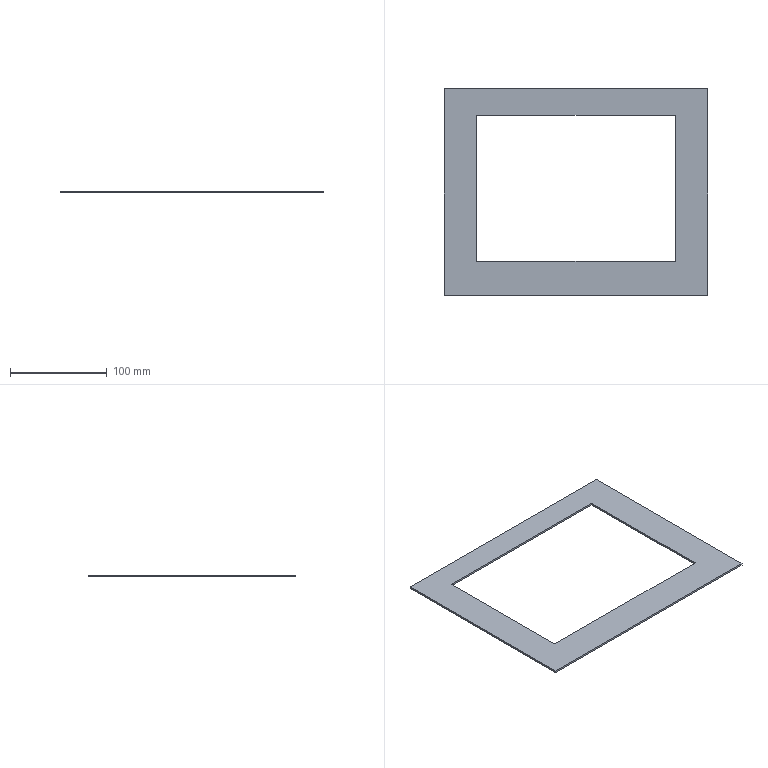Part | STEP file | Front guard plate SGN-7-05 | 1 solid | 10 faces | box 272 x 213 x 2 mm | volume 53962 mm3 | plane 10
STEP:
#1=CARTESIAN_POINT('',(0.,0.,0.));
#2=DIRECTION('',(0.,0.,1.));
#3=DIRECTION('',(1.,0.,0.));
#4=AXIS2_PLACEMENT_3D('',#1,#2,#3);
#5=CARTESIAN_POINT('',(136.,-106.5,0.));
#6=VERTEX_POINT('',#5);
#7=CARTESIAN_POINT('',(136.,106.5,0.));
#8=VERTEX_POINT('',#7);
#9=CARTESIAN_POINT('',(136.,-106.5,0.));
#10=DIRECTION('',(0.,1.,0.));
#11=VECTOR('',#10,1.);
#12=LINE('',#9,#11);
#13=CARTESIAN_POINT('',(136.,-106.5,-2.));
#14=DIRECTION('',(1.,0.,0.));
#15=DIRECTION('',(0.,0.,-1.));
#16=AXIS2_PLACEMENT_3D('',#13,#14,#15);
#17=PLANE('',#16);
#18=CARTESIAN_POINT('',(-2.,0.));
#19=DIRECTION('',(0.,1.));
#20=VECTOR('',#19,1.);
#21=LINE('',#18,#20);
#22=(GEOMETRIC_REPRESENTATION_CONTEXT(2)PARAMETRIC_REPRESENTATION_CONTEXT()REPRESENTATION_CONTEXT('',''));
#23=DEFINITIONAL_REPRESENTATION('',(#21),#22);
#24=PCURVE('',#17,#23);
#25=CARTESIAN_POINT('',(0.,0.,0.));
#26=DIRECTION('',(0.,0.,-1.));
#27=DIRECTION('',(-1.,0.,0.));
#28=AXIS2_PLACEMENT_3D('',#25,#26,#27);
#29=PLANE('',#28);
#30=CARTESIAN_POINT('',(-136.,-106.5));
#31=DIRECTION('',(0.,1.));
#32=VECTOR('',#31,1.);
#33=LINE('',#30,#32);
#34=(GEOMETRIC_REPRESENTATION_CONTEXT(2)PARAMETRIC_REPRESENTATION_CONTEXT()REPRESENTATION_CONTEXT('',''));
#35=DEFINITIONAL_REPRESENTATION('',(#33),#34);
#36=PCURVE('',#29,#35);
#37=SURFACE_CURVE('',#12,(#24,#36),.PCURVE_S1.);
#38=EDGE_CURVE('',#6,#8,#37,.T.);
#39=ORIENTED_EDGE('',*,*,#38,.F.);
#40=CARTESIAN_POINT('',(136.,-106.5,-2.));
#41=VERTEX_POINT('',#40);
#42=CARTESIAN_POINT('',(136.,-106.5,-2.));
#43=DIRECTION('',(0.,0.,1.));
#44=VECTOR('',#43,1.);
#45=LINE('',#42,#44);
#46=CARTESIAN_POINT('',(0.,0.));
#47=DIRECTION('',(-1.,0.));
#48=VECTOR('',#47,1.);
#49=LINE('',#46,#48);
#50=(GEOMETRIC_REPRESENTATION_CONTEXT(2)PARAMETRIC_REPRESENTATION_CONTEXT()REPRESENTATION_CONTEXT('',''));
#51=DEFINITIONAL_REPRESENTATION('',(#49),#50);
#52=PCURVE('',#17,#51);
#53=CARTESIAN_POINT('',(-136.,-106.5,-2.));
#54=DIRECTION('',(0.,-1.,0.));
#55=DIRECTION('',(0.,0.,-1.));
#56=AXIS2_PLACEMENT_3D('',#53,#54,#55);
#57=PLANE('',#56);
#58=CARTESIAN_POINT('',(0.,272.));
#59=DIRECTION('',(-1.,0.));
#60=VECTOR('',#59,1.);
#61=LINE('',#58,#60);
#62=(GEOMETRIC_REPRESENTATION_CONTEXT(2)PARAMETRIC_REPRESENTATION_CONTEXT()REPRESENTATION_CONTEXT('',''));
#63=DEFINITIONAL_REPRESENTATION('',(#61),#62);
#64=PCURVE('',#57,#63);
#65=SURFACE_CURVE('',#45,(#52,#64),.PCURVE_S1.);
#66=EDGE_CURVE('',#41,#6,#65,.T.);
#67=ORIENTED_EDGE('',*,*,#66,.F.);
#68=CARTESIAN_POINT('',(136.,106.5,-2.));
#69=VERTEX_POINT('',#68);
#70=CARTESIAN_POINT('',(136.,-106.5,-2.));
#71=DIRECTION('',(0.,1.,0.));
#72=VECTOR('',#71,1.);
#73=LINE('',#70,#72);
#74=CARTESIAN_POINT('',(0.,0.));
#75=DIRECTION('',(0.,1.));
#76=VECTOR('',#75,1.);
#77=LINE('',#74,#76);
#78=(GEOMETRIC_REPRESENTATION_CONTEXT(2)PARAMETRIC_REPRESENTATION_CONTEXT()REPRESENTATION_CONTEXT('',''));
#79=DEFINITIONAL_REPRESENTATION('',(#77),#78);
#80=PCURVE('',#17,#79);
#81=CARTESIAN_POINT('',(0.,0.,-2.));
#82=DIRECTION('',(0.,0.,-1.));
#83=DIRECTION('',(-1.,0.,0.));
#84=AXIS2_PLACEMENT_3D('',#81,#82,#83);
#85=PLANE('',#84);
#86=CARTESIAN_POINT('',(-136.,-106.5));
#87=DIRECTION('',(0.,1.));
#88=VECTOR('',#87,1.);
#89=LINE('',#86,#88);
#90=(GEOMETRIC_REPRESENTATION_CONTEXT(2)PARAMETRIC_REPRESENTATION_CONTEXT()REPRESENTATION_CONTEXT('',''));
#91=DEFINITIONAL_REPRESENTATION('',(#89),#90);
#92=PCURVE('',#85,#91);
#93=SURFACE_CURVE('',#73,(#80,#92),.PCURVE_S1.);
#94=EDGE_CURVE('',#41,#69,#93,.T.);
#95=ORIENTED_EDGE('',*,*,#94,.T.);
#96=CARTESIAN_POINT('',(136.,106.5,-2.));
#97=DIRECTION('',(0.,0.,1.));
#98=VECTOR('',#97,1.);
#99=LINE('',#96,#98);
#100=CARTESIAN_POINT('',(0.,213.));
#101=DIRECTION('',(-1.,0.));
#102=VECTOR('',#101,1.);
#103=LINE('',#100,#102);
#104=(GEOMETRIC_REPRESENTATION_CONTEXT(2)PARAMETRIC_REPRESENTATION_CONTEXT()REPRESENTATION_CONTEXT('',''));
#105=DEFINITIONAL_REPRESENTATION('',(#103),#104);
#106=PCURVE('',#17,#105);
#107=CARTESIAN_POINT('',(-136.,106.5,-2.));
#108=DIRECTION('',(0.,1.,0.));
#109=DIRECTION('',(0.,0.,1.));
#110=AXIS2_PLACEMENT_3D('',#107,#108,#109);
#111=PLANE('',#110);
#112=CARTESIAN_POINT('',(0.,272.));
#113=DIRECTION('',(1.,0.));
#114=VECTOR('',#113,1.);
#115=LINE('',#112,#114);
#116=(GEOMETRIC_REPRESENTATION_CONTEXT(2)PARAMETRIC_REPRESENTATION_CONTEXT()REPRESENTATION_CONTEXT('',''));
#117=DEFINITIONAL_REPRESENTATION('',(#115),#116);
#118=PCURVE('',#111,#117);
#119=SURFACE_CURVE('',#99,(#106,#118),.PCURVE_S1.);
#120=EDGE_CURVE('',#69,#8,#119,.T.);
#121=ORIENTED_EDGE('',*,*,#120,.T.);
#122=EDGE_LOOP('',(#39,#67,#95,#121));
#123=FACE_BOUND('',#122,.T.);
#124=ADVANCED_FACE('',(#123),#17,.T.);
#125=CARTESIAN_POINT('',(-136.,-106.5,0.));
#126=VERTEX_POINT('',#125);
#127=CARTESIAN_POINT('',(-136.,-106.5,0.));
#128=DIRECTION('',(1.,0.,0.));
#129=VECTOR('',#128,1.);
#130=LINE('',#127,#129);
#131=CARTESIAN_POINT('',(-2.,0.));
#132=DIRECTION('',(0.,1.));
#133=VECTOR('',#132,1.);
#134=LINE('',#131,#133);
#135=(GEOMETRIC_REPRESENTATION_CONTEXT(2)PARAMETRIC_REPRESENTATION_CONTEXT()REPRESENTATION_CONTEXT('',''));
#136=DEFINITIONAL_REPRESENTATION('',(#134),#135);
#137=PCURVE('',#57,#136);
#138=CARTESIAN_POINT('',(136.,-106.5));
#139=DIRECTION('',(-1.,0.));
#140=VECTOR('',#139,1.);
#141=LINE('',#138,#140);
#142=(GEOMETRIC_REPRESENTATION_CONTEXT(2)PARAMETRIC_REPRESENTATION_CONTEXT()REPRESENTATION_CONTEXT('',''));
#143=DEFINITIONAL_REPRESENTATION('',(#141),#142);
#144=PCURVE('',#29,#143);
#145=SURFACE_CURVE('',#130,(#137,#144),.PCURVE_S1.);
#146=EDGE_CURVE('',#126,#6,#145,.T.);
#147=ORIENTED_EDGE('',*,*,#146,.F.);
#148=CARTESIAN_POINT('',(-136.,-106.5,-2.));
#149=VERTEX_POINT('',#148);
#150=CARTESIAN_POINT('',(-136.,-106.5,-2.));
#151=DIRECTION('',(0.,0.,1.));
#152=VECTOR('',#151,1.);
#153=LINE('',#150,#152);
#154=CARTESIAN_POINT('',(0.,0.));
#155=DIRECTION('',(-1.,0.));
#156=VECTOR('',#155,1.);
#157=LINE('',#154,#156);
#158=(GEOMETRIC_REPRESENTATION_CONTEXT(2)PARAMETRIC_REPRESENTATION_CONTEXT()REPRESENTATION_CONTEXT('',''));
#159=DEFINITIONAL_REPRESENTATION('',(#157),#158);
#160=PCURVE('',#57,#159);
#161=CARTESIAN_POINT('',(-136.,-106.5,-2.));
#162=DIRECTION('',(-1.,0.,0.));
#163=DIRECTION('',(0.,0.,1.));
#164=AXIS2_PLACEMENT_3D('',#161,#162,#163);
#165=PLANE('',#164);
#166=CARTESIAN_POINT('',(0.,0.));
#167=DIRECTION('',(1.,0.));
#168=VECTOR('',#167,1.);
#169=LINE('',#166,#168);
#170=(GEOMETRIC_REPRESENTATION_CONTEXT(2)PARAMETRIC_REPRESENTATION_CONTEXT()REPRESENTATION_CONTEXT('',''));
#171=DEFINITIONAL_REPRESENTATION('',(#169),#170);
#172=PCURVE('',#165,#171);
#173=SURFACE_CURVE('',#153,(#160,#172),.PCURVE_S1.);
#174=EDGE_CURVE('',#149,#126,#173,.T.);
#175=ORIENTED_EDGE('',*,*,#174,.F.);
#176=CARTESIAN_POINT('',(-136.,-106.5,-2.));
#177=DIRECTION('',(1.,0.,0.));
#178=VECTOR('',#177,1.);
#179=LINE('',#176,#178);
#180=CARTESIAN_POINT('',(0.,0.));
#181=DIRECTION('',(0.,1.));
#182=VECTOR('',#181,1.);
#183=LINE('',#180,#182);
#184=(GEOMETRIC_REPRESENTATION_CONTEXT(2)PARAMETRIC_REPRESENTATION_CONTEXT()REPRESENTATION_CONTEXT('',''));
#185=DEFINITIONAL_REPRESENTATION('',(#183),#184);
#186=PCURVE('',#57,#185);
#187=CARTESIAN_POINT('',(136.,-106.5));
#188=DIRECTION('',(-1.,0.));
#189=VECTOR('',#188,1.);
#190=LINE('',#187,#189);
#191=(GEOMETRIC_REPRESENTATION_CONTEXT(2)PARAMETRIC_REPRESENTATION_CONTEXT()REPRESENTATION_CONTEXT('',''));
#192=DEFINITIONAL_REPRESENTATION('',(#190),#191);
#193=PCURVE('',#85,#192);
#194=SURFACE_CURVE('',#179,(#186,#193),.PCURVE_S1.);
#195=EDGE_CURVE('',#149,#41,#194,.T.);
#196=ORIENTED_EDGE('',*,*,#195,.T.);
#197=ORIENTED_EDGE('',*,*,#66,.T.);
#198=EDGE_LOOP('',(#147,#175,#196,#197));
#199=FACE_BOUND('',#198,.T.);
#200=ADVANCED_FACE('',(#199),#57,.T.);
#201=CARTESIAN_POINT('',(-136.,106.5,0.));
#202=VERTEX_POINT('',#201);
#203=CARTESIAN_POINT('',(-136.,-106.5,0.));
#204=DIRECTION('',(0.,-1.,0.));
#205=VECTOR('',#204,1.);
#206=LINE('',#203,#205);
#207=CARTESIAN_POINT('',(2.,0.));
#208=DIRECTION('',(0.,-1.));
#209=VECTOR('',#208,1.);
#210=LINE('',#207,#209);
#211=(GEOMETRIC_REPRESENTATION_CONTEXT(2)PARAMETRIC_REPRESENTATION_CONTEXT()REPRESENTATION_CONTEXT('',''));
#212=DEFINITIONAL_REPRESENTATION('',(#210),#211);
#213=PCURVE('',#165,#212);
#214=CARTESIAN_POINT('',(136.,-106.5));
#215=DIRECTION('',(0.,-1.));
#216=VECTOR('',#215,1.);
#217=LINE('',#214,#216);
#218=(GEOMETRIC_REPRESENTATION_CONTEXT(2)PARAMETRIC_REPRESENTATION_CONTEXT()REPRESENTATION_CONTEXT('',''));
#219=DEFINITIONAL_REPRESENTATION('',(#217),#218);
#220=PCURVE('',#29,#219);
#221=SURFACE_CURVE('',#206,(#213,#220),.PCURVE_S1.);
#222=EDGE_CURVE('',#202,#126,#221,.T.);
#223=ORIENTED_EDGE('',*,*,#222,.F.);
#224=CARTESIAN_POINT('',(-136.,106.5,-2.));
#225=VERTEX_POINT('',#224);
#226=CARTESIAN_POINT('',(-136.,106.5,-2.));
#227=DIRECTION('',(0.,0.,1.));
#228=VECTOR('',#227,1.);
#229=LINE('',#226,#228);
#230=CARTESIAN_POINT('',(0.,213.));
#231=DIRECTION('',(1.,0.));
#232=VECTOR('',#231,1.);
#233=LINE('',#230,#232);
#234=(GEOMETRIC_REPRESENTATION_CONTEXT(2)PARAMETRIC_REPRESENTATION_CONTEXT()REPRESENTATION_CONTEXT('',''));
#235=DEFINITIONAL_REPRESENTATION('',(#233),#234);
#236=PCURVE('',#165,#235);
#237=CARTESIAN_POINT('',(0.,0.));
#238=DIRECTION('',(1.,0.));
#239=VECTOR('',#238,1.);
#240=LINE('',#237,#239);
#241=(GEOMETRIC_REPRESENTATION_CONTEXT(2)PARAMETRIC_REPRESENTATION_CONTEXT()REPRESENTATION_CONTEXT('',''));
#242=DEFINITIONAL_REPRESENTATION('',(#240),#241);
#243=PCURVE('',#111,#242);
#244=SURFACE_CURVE('',#229,(#236,#243),.PCURVE_S1.);
#245=EDGE_CURVE('',#225,#202,#244,.T.);
#246=ORIENTED_EDGE('',*,*,#245,.F.);
#247=CARTESIAN_POINT('',(-136.,-106.5,-2.));
#248=DIRECTION('',(0.,-1.,0.));
#249=VECTOR('',#248,1.);
#250=LINE('',#247,#249);
#251=CARTESIAN_POINT('',(0.,0.));
#252=DIRECTION('',(0.,-1.));
#253=VECTOR('',#252,1.);
#254=LINE('',#251,#253);
#255=(GEOMETRIC_REPRESENTATION_CONTEXT(2)PARAMETRIC_REPRESENTATION_CONTEXT()REPRESENTATION_CONTEXT('',''));
#256=DEFINITIONAL_REPRESENTATION('',(#254),#255);
#257=PCURVE('',#165,#256);
#258=CARTESIAN_POINT('',(136.,-106.5));
#259=DIRECTION('',(0.,-1.));
#260=VECTOR('',#259,1.);
#261=LINE('',#258,#260);
#262=(GEOMETRIC_REPRESENTATION_CONTEXT(2)PARAMETRIC_REPRESENTATION_CONTEXT()REPRESENTATION_CONTEXT('',''));
#263=DEFINITIONAL_REPRESENTATION('',(#261),#262);
#264=PCURVE('',#85,#263);
#265=SURFACE_CURVE('',#250,(#257,#264),.PCURVE_S1.);
#266=EDGE_CURVE('',#225,#149,#265,.T.);
#267=ORIENTED_EDGE('',*,*,#266,.T.);
#268=ORIENTED_EDGE('',*,*,#174,.T.);
#269=EDGE_LOOP('',(#223,#246,#267,#268));
#270=FACE_BOUND('',#269,.T.);
#271=ADVANCED_FACE('',(#270),#165,.T.);
#272=CARTESIAN_POINT('',(-136.,106.5,0.));
#273=DIRECTION('',(-1.,0.,0.));
#274=VECTOR('',#273,1.);
#275=LINE('',#272,#274);
#276=CARTESIAN_POINT('',(2.,0.));
#277=DIRECTION('',(0.,-1.));
#278=VECTOR('',#277,1.);
#279=LINE('',#276,#278);
#280=(GEOMETRIC_REPRESENTATION_CONTEXT(2)PARAMETRIC_REPRESENTATION_CONTEXT()REPRESENTATION_CONTEXT('',''));
#281=DEFINITIONAL_REPRESENTATION('',(#279),#280);
#282=PCURVE('',#111,#281);
#283=CARTESIAN_POINT('',(136.,106.5));
#284=DIRECTION('',(1.,0.));
#285=VECTOR('',#284,1.);
#286=LINE('',#283,#285);
#287=(GEOMETRIC_REPRESENTATION_CONTEXT(2)PARAMETRIC_REPRESENTATION_CONTEXT()REPRESENTATION_CONTEXT('',''));
#288=DEFINITIONAL_REPRESENTATION('',(#286),#287);
#289=PCURVE('',#29,#288);
#290=SURFACE_CURVE('',#275,(#282,#289),.PCURVE_S1.);
#291=EDGE_CURVE('',#8,#202,#290,.T.);
#292=ORIENTED_EDGE('',*,*,#291,.F.);
#293=ORIENTED_EDGE('',*,*,#120,.F.);
#294=CARTESIAN_POINT('',(-136.,106.5,-2.));
#295=DIRECTION('',(-1.,0.,0.));
#296=VECTOR('',#295,1.);
#297=LINE('',#294,#296);
#298=CARTESIAN_POINT('',(0.,0.));
#299=DIRECTION('',(0.,-1.));
#300=VECTOR('',#299,1.);
#301=LINE('',#298,#300);
#302=(GEOMETRIC_REPRESENTATION_CONTEXT(2)PARAMETRIC_REPRESENTATION_CONTEXT()REPRESENTATION_CONTEXT('',''));
#303=DEFINITIONAL_REPRESENTATION('',(#301),#302);
#304=PCURVE('',#111,#303);
#305=CARTESIAN_POINT('',(136.,106.5));
#306=DIRECTION('',(1.,0.));
#307=VECTOR('',#306,1.);
#308=LINE('',#305,#307);
#309=(GEOMETRIC_REPRESENTATION_CONTEXT(2)PARAMETRIC_REPRESENTATION_CONTEXT()REPRESENTATION_CONTEXT('',''));
#310=DEFINITIONAL_REPRESENTATION('',(#308),#309);
#311=PCURVE('',#85,#310);
#312=SURFACE_CURVE('',#297,(#304,#311),.PCURVE_S1.);
#313=EDGE_CURVE('',#69,#225,#312,.T.);
#314=ORIENTED_EDGE('',*,*,#313,.T.);
#315=ORIENTED_EDGE('',*,*,#245,.T.);
#316=EDGE_LOOP('',(#292,#293,#314,#315));
#317=FACE_BOUND('',#316,.T.);
#318=ADVANCED_FACE('',(#317),#111,.T.);
#319=CARTESIAN_POINT('',(-102.5,-71.5,-2.));
#320=VERTEX_POINT('',#319);
#321=CARTESIAN_POINT('',(-102.5,79.5,-2.));
#322=VERTEX_POINT('',#321);
#323=CARTESIAN_POINT('',(-102.5,0.,-2.));
#324=DIRECTION('',(0.,1.,0.));
#325=VECTOR('',#324,1.);
#326=LINE('',#323,#325);
#327=CARTESIAN_POINT('',(102.5,0.));
#328=DIRECTION('',(0.,1.));
#329=VECTOR('',#328,1.);
#330=LINE('',#327,#329);
#331=(GEOMETRIC_REPRESENTATION_CONTEXT(2)PARAMETRIC_REPRESENTATION_CONTEXT()REPRESENTATION_CONTEXT('',''));
#332=DEFINITIONAL_REPRESENTATION('',(#330),#331);
#333=PCURVE('',#85,#332);
#334=CARTESIAN_POINT('',(-102.5,79.5,-10.));
#335=DIRECTION('',(-1.,0.,0.));
#336=DIRECTION('',(0.,-1.,0.));
#337=AXIS2_PLACEMENT_3D('',#334,#335,#336);
#338=PLANE('',#337);
#339=CARTESIAN_POINT('',(79.5,8.));
#340=DIRECTION('',(-1.,0.));
#341=VECTOR('',#340,1.);
#342=LINE('',#339,#341);
#343=(GEOMETRIC_REPRESENTATION_CONTEXT(2)PARAMETRIC_REPRESENTATION_CONTEXT()REPRESENTATION_CONTEXT('',''));
#344=DEFINITIONAL_REPRESENTATION('',(#342),#343);
#345=PCURVE('',#338,#344);
#346=SURFACE_CURVE('',#326,(#333,#345),.PCURVE_S1.);
#347=EDGE_CURVE('',#320,#322,#346,.T.);
#348=ORIENTED_EDGE('',*,*,#347,.F.);
#349=CARTESIAN_POINT('',(102.5,-71.5,-2.));
#350=VERTEX_POINT('',#349);
#351=CARTESIAN_POINT('',(0.,-71.5,-2.));
#352=DIRECTION('',(-1.,0.,0.));
#353=VECTOR('',#352,1.);
#354=LINE('',#351,#353);
#355=CARTESIAN_POINT('',(0.,-71.5));
#356=DIRECTION('',(1.,0.));
#357=VECTOR('',#356,1.);
#358=LINE('',#355,#357);
#359=(GEOMETRIC_REPRESENTATION_CONTEXT(2)PARAMETRIC_REPRESENTATION_CONTEXT()REPRESENTATION_CONTEXT('',''));
#360=DEFINITIONAL_REPRESENTATION('',(#358),#359);
#361=PCURVE('',#85,#360);
#362=CARTESIAN_POINT('',(-102.5,-71.5,-10.));
#363=DIRECTION('',(0.,-1.,0.));
#364=DIRECTION('',(0.,0.,-1.));
#365=AXIS2_PLACEMENT_3D('',#362,#363,#364);
#366=PLANE('',#365);
#367=CARTESIAN_POINT('',(-8.,102.5));
#368=DIRECTION('',(0.,-1.));
#369=VECTOR('',#368,1.);
#370=LINE('',#367,#369);
#371=(GEOMETRIC_REPRESENTATION_CONTEXT(2)PARAMETRIC_REPRESENTATION_CONTEXT()REPRESENTATION_CONTEXT('',''));
#372=DEFINITIONAL_REPRESENTATION('',(#370),#371);
#373=PCURVE('',#366,#372);
#374=SURFACE_CURVE('',#354,(#361,#373),.PCURVE_S1.);
#375=EDGE_CURVE('',#350,#320,#374,.T.);
#376=ORIENTED_EDGE('',*,*,#375,.F.);
#377=CARTESIAN_POINT('',(102.5,79.5,-2.));
#378=VERTEX_POINT('',#377);
#379=CARTESIAN_POINT('',(102.5,0.,-2.));
#380=DIRECTION('',(0.,1.,0.));
#381=VECTOR('',#380,1.);
#382=LINE('',#379,#381);
#383=CARTESIAN_POINT('',(-102.5,0.));
#384=DIRECTION('',(0.,1.));
#385=VECTOR('',#384,1.);
#386=LINE('',#383,#385);
#387=(GEOMETRIC_REPRESENTATION_CONTEXT(2)PARAMETRIC_REPRESENTATION_CONTEXT()REPRESENTATION_CONTEXT('',''));
#388=DEFINITIONAL_REPRESENTATION('',(#386),#387);
#389=PCURVE('',#85,#388);
#390=CARTESIAN_POINT('',(102.5,79.5,-10.));
#391=DIRECTION('',(-1.,0.,0.));
#392=DIRECTION('',(0.,-1.,0.));
#393=AXIS2_PLACEMENT_3D('',#390,#391,#392);
#394=PLANE('',#393);
#395=CARTESIAN_POINT('',(79.5,8.));
#396=DIRECTION('',(-1.,0.));
#397=VECTOR('',#396,1.);
#398=LINE('',#395,#397);
#399=(GEOMETRIC_REPRESENTATION_CONTEXT(2)PARAMETRIC_REPRESENTATION_CONTEXT()REPRESENTATION_CONTEXT('',''));
#400=DEFINITIONAL_REPRESENTATION('',(#398),#399);
#401=PCURVE('',#394,#400);
#402=SURFACE_CURVE('',#382,(#389,#401),.PCURVE_S1.);
#403=EDGE_CURVE('',#350,#378,#402,.T.);
#404=ORIENTED_EDGE('',*,*,#403,.T.);
#405=CARTESIAN_POINT('',(0.,79.5,-2.));
#406=DIRECTION('',(-1.,0.,0.));
#407=VECTOR('',#406,1.);
#408=LINE('',#405,#407);
#409=CARTESIAN_POINT('',(0.,79.5));
#410=DIRECTION('',(1.,0.));
#411=VECTOR('',#410,1.);
#412=LINE('',#409,#411);
#413=(GEOMETRIC_REPRESENTATION_CONTEXT(2)PARAMETRIC_REPRESENTATION_CONTEXT()REPRESENTATION_CONTEXT('',''));
#414=DEFINITIONAL_REPRESENTATION('',(#412),#413);
#415=PCURVE('',#85,#414);
#416=CARTESIAN_POINT('',(-102.5,79.5,-10.));
#417=DIRECTION('',(0.,-1.,0.));
#418=DIRECTION('',(0.,0.,-1.));
#419=AXIS2_PLACEMENT_3D('',#416,#417,#418);
#420=PLANE('',#419);
#421=CARTESIAN_POINT('',(-8.,102.5));
#422=DIRECTION('',(0.,-1.));
#423=VECTOR('',#422,1.);
#424=LINE('',#421,#423);
#425=(GEOMETRIC_REPRESENTATION_CONTEXT(2)PARAMETRIC_REPRESENTATION_CONTEXT()REPRESENTATION_CONTEXT('',''));
#426=DEFINITIONAL_REPRESENTATION('',(#424),#425);
#427=PCURVE('',#420,#426);
#428=SURFACE_CURVE('',#408,(#415,#427),.PCURVE_S1.);
#429=EDGE_CURVE('',#378,#322,#428,.T.);
#430=ORIENTED_EDGE('',*,*,#429,.T.);
#431=EDGE_LOOP('',(#348,#376,#404,#430));
#432=FACE_BOUND('',#431,.T.);
#433=ORIENTED_EDGE('',*,*,#94,.F.);
#434=ORIENTED_EDGE('',*,*,#195,.F.);
#435=ORIENTED_EDGE('',*,*,#266,.F.);
#436=ORIENTED_EDGE('',*,*,#313,.F.);
#437=EDGE_LOOP('',(#433,#434,#435,#436));
#438=FACE_BOUND('',#437,.T.);
#439=ADVANCED_FACE('',(#432,#438),#85,.T.);
#440=CARTESIAN_POINT('',(-102.5,-71.5,0.));
#441=VERTEX_POINT('',#440);
#442=CARTESIAN_POINT('',(102.5,-71.5,0.));
#443=VERTEX_POINT('',#442);
#444=CARTESIAN_POINT('',(-102.5,-71.5,0.));
#445=DIRECTION('',(1.,0.,0.));
#446=VECTOR('',#445,1.);
#447=LINE('',#444,#446);
#448=CARTESIAN_POINT('',(102.5,-71.5));
#449=DIRECTION('',(-1.,0.));
#450=VECTOR('',#449,1.);
#451=LINE('',#448,#450);
#452=(GEOMETRIC_REPRESENTATION_CONTEXT(2)PARAMETRIC_REPRESENTATION_CONTEXT()REPRESENTATION_CONTEXT('',''));
#453=DEFINITIONAL_REPRESENTATION('',(#451),#452);
#454=PCURVE('',#29,#453);
#455=CARTESIAN_POINT('',(-10.,0.));
#456=DIRECTION('',(0.,1.));
#457=VECTOR('',#456,1.);
#458=LINE('',#455,#457);
#459=(GEOMETRIC_REPRESENTATION_CONTEXT(2)PARAMETRIC_REPRESENTATION_CONTEXT()REPRESENTATION_CONTEXT('',''));
#460=DEFINITIONAL_REPRESENTATION('',(#458),#459);
#461=PCURVE('',#366,#460);
#462=SURFACE_CURVE('',#447,(#454,#461),.PCURVE_S1.);
#463=EDGE_CURVE('',#441,#443,#462,.T.);
#464=ORIENTED_EDGE('',*,*,#463,.F.);
#465=CARTESIAN_POINT('',(-102.5,79.5,0.));
#466=VERTEX_POINT('',#465);
#467=CARTESIAN_POINT('',(-102.5,79.5,0.));
#468=DIRECTION('',(0.,-1.,0.));
#469=VECTOR('',#468,1.);
#470=LINE('',#467,#469);
#471=CARTESIAN_POINT('',(102.5,79.5));
#472=DIRECTION('',(0.,-1.));
#473=VECTOR('',#472,1.);
#474=LINE('',#471,#473);
#475=(GEOMETRIC_REPRESENTATION_CONTEXT(2)PARAMETRIC_REPRESENTATION_CONTEXT()REPRESENTATION_CONTEXT('',''));
#476=DEFINITIONAL_REPRESENTATION('',(#474),#475);
#477=PCURVE('',#29,#476);
#478=CARTESIAN_POINT('',(0.,10.));
#479=DIRECTION('',(1.,0.));
#480=VECTOR('',#479,1.);
#481=LINE('',#478,#480);
#482=(GEOMETRIC_REPRESENTATION_CONTEXT(2)PARAMETRIC_REPRESENTATION_CONTEXT()REPRESENTATION_CONTEXT('',''));
#483=DEFINITIONAL_REPRESENTATION('',(#481),#482);
#484=PCURVE('',#338,#483);
#485=SURFACE_CURVE('',#470,(#477,#484),.PCURVE_S1.);
#486=EDGE_CURVE('',#466,#441,#485,.T.);
#487=ORIENTED_EDGE('',*,*,#486,.F.);
#488=CARTESIAN_POINT('',(102.5,79.5,0.));
#489=VERTEX_POINT('',#488);
#490=CARTESIAN_POINT('',(-102.5,79.5,0.));
#491=DIRECTION('',(1.,0.,0.));
#492=VECTOR('',#491,1.);
#493=LINE('',#490,#492);
#494=CARTESIAN_POINT('',(102.5,79.5));
#495=DIRECTION('',(-1.,0.));
#496=VECTOR('',#495,1.);
#497=LINE('',#494,#496);
#498=(GEOMETRIC_REPRESENTATION_CONTEXT(2)PARAMETRIC_REPRESENTATION_CONTEXT()REPRESENTATION_CONTEXT('',''));
#499=DEFINITIONAL_REPRESENTATION('',(#497),#498);
#500=PCURVE('',#29,#499);
#501=CARTESIAN_POINT('',(-10.,0.));
#502=DIRECTION('',(0.,1.));
#503=VECTOR('',#502,1.);
#504=LINE('',#501,#503);
#505=(GEOMETRIC_REPRESENTATION_CONTEXT(2)PARAMETRIC_REPRESENTATION_CONTEXT()REPRESENTATION_CONTEXT('',''));
#506=DEFINITIONAL_REPRESENTATION('',(#504),#505);
#507=PCURVE('',#420,#506);
#508=SURFACE_CURVE('',#493,(#500,#507),.PCURVE_S1.);
#509=EDGE_CURVE('',#466,#489,#508,.T.);
#510=ORIENTED_EDGE('',*,*,#509,.T.);
#511=CARTESIAN_POINT('',(102.5,79.5,0.));
#512=DIRECTION('',(0.,-1.,0.));
#513=VECTOR('',#512,1.);
#514=LINE('',#511,#513);
#515=CARTESIAN_POINT('',(-102.5,79.5));
#516=DIRECTION('',(0.,-1.));
#517=VECTOR('',#516,1.);
#518=LINE('',#515,#517);
#519=(GEOMETRIC_REPRESENTATION_CONTEXT(2)PARAMETRIC_REPRESENTATION_CONTEXT()REPRESENTATION_CONTEXT('',''));
#520=DEFINITIONAL_REPRESENTATION('',(#518),#519);
#521=PCURVE('',#29,#520);
#522=CARTESIAN_POINT('',(0.,10.));
#523=DIRECTION('',(1.,0.));
#524=VECTOR('',#523,1.);
#525=LINE('',#522,#524);
#526=(GEOMETRIC_REPRESENTATION_CONTEXT(2)PARAMETRIC_REPRESENTATION_CONTEXT()REPRESENTATION_CONTEXT('',''));
#527=DEFINITIONAL_REPRESENTATION('',(#525),#526);
#528=PCURVE('',#394,#527);
#529=SURFACE_CURVE('',#514,(#521,#528),.PCURVE_S1.);
#530=EDGE_CURVE('',#489,#443,#529,.T.);
#531=ORIENTED_EDGE('',*,*,#530,.T.);
#532=EDGE_LOOP('',(#464,#487,#510,#531));
#533=FACE_BOUND('',#532,.T.);
#534=ORIENTED_EDGE('',*,*,#38,.T.);
#535=ORIENTED_EDGE('',*,*,#291,.T.);
#536=ORIENTED_EDGE('',*,*,#222,.T.);
#537=ORIENTED_EDGE('',*,*,#146,.T.);
#538=EDGE_LOOP('',(#534,#535,#536,#537));
#539=FACE_BOUND('',#538,.T.);
#540=ADVANCED_FACE('',(#533,#539),#29,.F.);
#541=ORIENTED_EDGE('',*,*,#347,.T.);
#542=CARTESIAN_POINT('',(-102.5,79.5,-10.));
#543=DIRECTION('',(0.,0.,1.));
#544=VECTOR('',#543,1.);
#545=LINE('',#542,#544);
#546=CARTESIAN_POINT('',(0.,0.));
#547=DIRECTION('',(0.,1.));
#548=VECTOR('',#547,1.);
#549=LINE('',#546,#548);
#550=(GEOMETRIC_REPRESENTATION_CONTEXT(2)PARAMETRIC_REPRESENTATION_CONTEXT()REPRESENTATION_CONTEXT('',''));
#551=DEFINITIONAL_REPRESENTATION('',(#549),#550);
#552=PCURVE('',#338,#551);
#553=CARTESIAN_POINT('',(0.,0.));
#554=DIRECTION('',(-1.,0.));
#555=VECTOR('',#554,1.);
#556=LINE('',#553,#555);
#557=(GEOMETRIC_REPRESENTATION_CONTEXT(2)PARAMETRIC_REPRESENTATION_CONTEXT()REPRESENTATION_CONTEXT('',''));
#558=DEFINITIONAL_REPRESENTATION('',(#556),#557);
#559=PCURVE('',#420,#558);
#560=SURFACE_CURVE('',#545,(#552,#559),.PCURVE_S1.);
#561=EDGE_CURVE('',#322,#466,#560,.T.);
#562=ORIENTED_EDGE('',*,*,#561,.T.);
#563=ORIENTED_EDGE('',*,*,#486,.T.);
#564=CARTESIAN_POINT('',(-102.5,-71.5,-10.));
#565=DIRECTION('',(0.,0.,1.));
#566=VECTOR('',#565,1.);
#567=LINE('',#564,#566);
#568=CARTESIAN_POINT('',(151.,0.));
#569=DIRECTION('',(0.,1.));
#570=VECTOR('',#569,1.);
#571=LINE('',#568,#570);
#572=(GEOMETRIC_REPRESENTATION_CONTEXT(2)PARAMETRIC_REPRESENTATION_CONTEXT()REPRESENTATION_CONTEXT('',''));
#573=DEFINITIONAL_REPRESENTATION('',(#571),#572);
#574=PCURVE('',#338,#573);
#575=CARTESIAN_POINT('',(0.,0.));
#576=DIRECTION('',(-1.,0.));
#577=VECTOR('',#576,1.);
#578=LINE('',#575,#577);
#579=(GEOMETRIC_REPRESENTATION_CONTEXT(2)PARAMETRIC_REPRESENTATION_CONTEXT()REPRESENTATION_CONTEXT('',''));
#580=DEFINITIONAL_REPRESENTATION('',(#578),#579);
#581=PCURVE('',#366,#580);
#582=SURFACE_CURVE('',#567,(#574,#581),.PCURVE_S1.);
#583=EDGE_CURVE('',#320,#441,#582,.T.);
#584=ORIENTED_EDGE('',*,*,#583,.F.);
#585=EDGE_LOOP('',(#541,#562,#563,#584));
#586=FACE_BOUND('',#585,.T.);
#587=ADVANCED_FACE('',(#586),#338,.F.);
#588=CARTESIAN_POINT('',(102.5,79.5,-10.));
#589=DIRECTION('',(0.,0.,1.));
#590=VECTOR('',#589,1.);
#591=LINE('',#588,#590);
#592=CARTESIAN_POINT('',(0.,205.));
#593=DIRECTION('',(-1.,0.));
#594=VECTOR('',#593,1.);
#595=LINE('',#592,#594);
#596=(GEOMETRIC_REPRESENTATION_CONTEXT(2)PARAMETRIC_REPRESENTATION_CONTEXT()REPRESENTATION_CONTEXT('',''));
#597=DEFINITIONAL_REPRESENTATION('',(#595),#596);
#598=PCURVE('',#420,#597);
#599=CARTESIAN_POINT('',(0.,0.));
#600=DIRECTION('',(0.,1.));
#601=VECTOR('',#600,1.);
#602=LINE('',#599,#601);
#603=(GEOMETRIC_REPRESENTATION_CONTEXT(2)PARAMETRIC_REPRESENTATION_CONTEXT()REPRESENTATION_CONTEXT('',''));
#604=DEFINITIONAL_REPRESENTATION('',(#602),#603);
#605=PCURVE('',#394,#604);
#606=SURFACE_CURVE('',#591,(#598,#605),.PCURVE_S1.);
#607=EDGE_CURVE('',#378,#489,#606,.T.);
#608=ORIENTED_EDGE('',*,*,#607,.T.);
#609=ORIENTED_EDGE('',*,*,#509,.F.);
#610=ORIENTED_EDGE('',*,*,#561,.F.);
#611=ORIENTED_EDGE('',*,*,#429,.F.);
#612=EDGE_LOOP('',(#608,#609,#610,#611));
#613=FACE_BOUND('',#612,.T.);
#614=ADVANCED_FACE('',(#613),#420,.T.);
#615=CARTESIAN_POINT('',(102.5,-71.5,-10.));
#616=DIRECTION('',(0.,0.,1.));
#617=VECTOR('',#616,1.);
#618=LINE('',#615,#617);
#619=CARTESIAN_POINT('',(151.,0.));
#620=DIRECTION('',(0.,1.));
#621=VECTOR('',#620,1.);
#622=LINE('',#619,#621);
#623=(GEOMETRIC_REPRESENTATION_CONTEXT(2)PARAMETRIC_REPRESENTATION_CONTEXT()REPRESENTATION_CONTEXT('',''));
#624=DEFINITIONAL_REPRESENTATION('',(#622),#623);
#625=PCURVE('',#394,#624);
#626=CARTESIAN_POINT('',(0.,205.));
#627=DIRECTION('',(-1.,0.));
#628=VECTOR('',#627,1.);
#629=LINE('',#626,#628);
#630=(GEOMETRIC_REPRESENTATION_CONTEXT(2)PARAMETRIC_REPRESENTATION_CONTEXT()REPRESENTATION_CONTEXT('',''));
#631=DEFINITIONAL_REPRESENTATION('',(#629),#630);
#632=PCURVE('',#366,#631);
#633=SURFACE_CURVE('',#618,(#625,#632),.PCURVE_S1.);
#634=EDGE_CURVE('',#350,#443,#633,.T.);
#635=ORIENTED_EDGE('',*,*,#634,.T.);
#636=ORIENTED_EDGE('',*,*,#530,.F.);
#637=ORIENTED_EDGE('',*,*,#607,.F.);
#638=ORIENTED_EDGE('',*,*,#403,.F.);
#639=EDGE_LOOP('',(#635,#636,#637,#638));
#640=FACE_BOUND('',#639,.T.);
#641=ADVANCED_FACE('',(#640),#394,.T.);
#642=ORIENTED_EDGE('',*,*,#375,.T.);
#643=ORIENTED_EDGE('',*,*,#583,.T.);
#644=ORIENTED_EDGE('',*,*,#463,.T.);
#645=ORIENTED_EDGE('',*,*,#634,.F.);
#646=EDGE_LOOP('',(#642,#643,#644,#645));
#647=FACE_BOUND('',#646,.T.);
#648=ADVANCED_FACE('',(#647),#366,.F.);
#649=CLOSED_SHELL('',(#124,#200,#271,#318,#439,#540,#587,#614,#641,#648));
#650=MANIFOLD_SOLID_BREP('',#649);
#651=(LENGTH_UNIT()NAMED_UNIT(*)SI_UNIT(.MILLI.,.METRE.));
#652=UNCERTAINTY_MEASURE_WITH_UNIT(LENGTH_MEASURE(0.0000001),#651,'','');
#653=(NAMED_UNIT(*)PLANE_ANGLE_UNIT()SI_UNIT($,.RADIAN.));
#654=(NAMED_UNIT(*)SI_UNIT($,.STERADIAN.)SOLID_ANGLE_UNIT());
#655=(GEOMETRIC_REPRESENTATION_CONTEXT(3)GLOBAL_UNCERTAINTY_ASSIGNED_CONTEXT((#652))GLOBAL_UNIT_ASSIGNED_CONTEXT((#651,#653,#654))REPRESENTATION_CONTEXT('',''));
#656=ADVANCED_BREP_SHAPE_REPRESENTATION('',(#4,#650),#655);